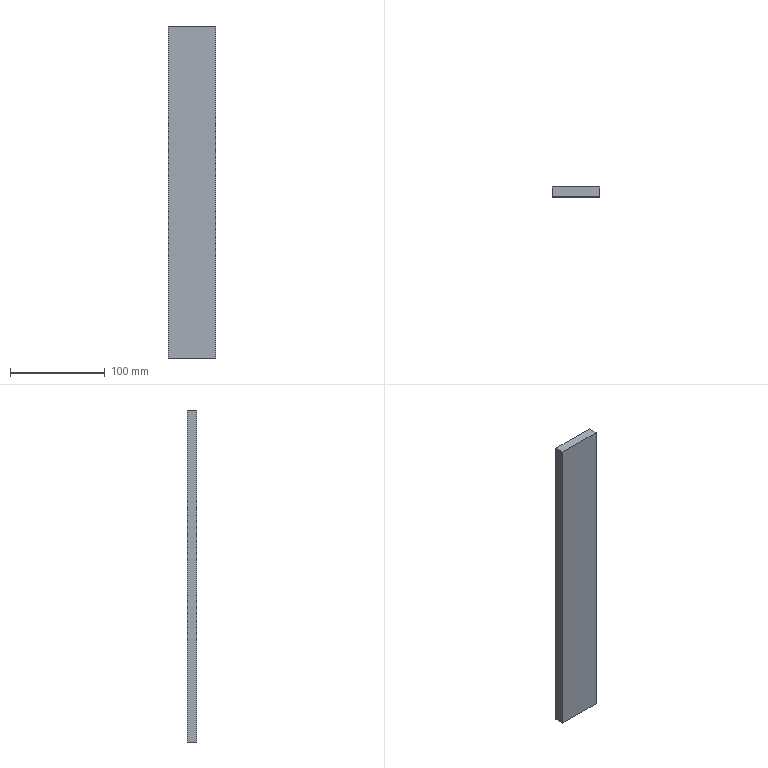Part | NX | features solid 2 | 1 solid | 6 faces | box 50 x 10 x 350 mm | volume 175000 mm3 | plane 6
STEP:
#1=CARTESIAN_POINT('',(635.,615.,-175.));
#2=VERTEX_POINT('',#1);
#3=CARTESIAN_POINT('',(635.,625.,-175.));
#4=VERTEX_POINT('',#3);
#5=CARTESIAN_POINT('',(635.,615.,-175.));
#6=DIRECTION('',(0.,-1.,0.));
#7=VECTOR('',#6,1000.);
#8=LINE('',#5,#7);
#9=EDGE_CURVE('',#2,#4,#8,.F.);
#10=ORIENTED_EDGE('',*,*,#9,.F.);
#11=CARTESIAN_POINT('',(635.,615.,175.));
#12=VERTEX_POINT('',#11);
#13=CARTESIAN_POINT('',(635.,615.,-165.));
#14=DIRECTION('',(0.,0.,1.));
#15=VECTOR('',#14,1000.);
#16=LINE('',#13,#15);
#17=EDGE_CURVE('',#2,#12,#16,.T.);
#18=ORIENTED_EDGE('',*,*,#17,.T.);
#19=CARTESIAN_POINT('',(635.,625.,175.));
#20=VERTEX_POINT('',#19);
#21=CARTESIAN_POINT('',(635.,615.,175.));
#22=DIRECTION('',(0.,1.,0.));
#23=VECTOR('',#22,1000.);
#24=LINE('',#21,#23);
#25=EDGE_CURVE('',#12,#20,#24,.T.);
#26=ORIENTED_EDGE('',*,*,#25,.T.);
#27=CARTESIAN_POINT('',(635.,625.,-165.));
#28=DIRECTION('',(0.,0.,-1.));
#29=VECTOR('',#28,1000.);
#30=LINE('',#27,#29);
#31=EDGE_CURVE('',#4,#20,#30,.F.);
#32=ORIENTED_EDGE('',*,*,#31,.F.);
#33=EDGE_LOOP('',(#10,#18,#26,#32));
#34=FACE_BOUND('',#33,.T.);
#35=CARTESIAN_POINT('',(635.,615.,-165.));
#36=DIRECTION('',(-1.,0.,0.));
#37=DIRECTION('',(0.,0.,1.));
#38=AXIS2_PLACEMENT_3D('',#35,#36,#37);
#39=PLANE('',#38);
#40=ADVANCED_FACE('',(#34),#39,.T.);
#41=ORIENTED_EDGE('',*,*,#25,.F.);
#42=CARTESIAN_POINT('',(685.,615.,175.));
#43=VERTEX_POINT('',#42);
#44=CARTESIAN_POINT('',(635.,615.,175.));
#45=DIRECTION('',(1.,0.,0.));
#46=VECTOR('',#45,1000.);
#47=LINE('',#44,#46);
#48=EDGE_CURVE('',#12,#43,#47,.T.);
#49=ORIENTED_EDGE('',*,*,#48,.T.);
#50=CARTESIAN_POINT('',(685.,625.,175.));
#51=VERTEX_POINT('',#50);
#52=CARTESIAN_POINT('',(685.,615.,175.));
#53=DIRECTION('',(0.,-1.,0.));
#54=VECTOR('',#53,1000.);
#55=LINE('',#52,#54);
#56=EDGE_CURVE('',#43,#51,#55,.F.);
#57=ORIENTED_EDGE('',*,*,#56,.T.);
#58=CARTESIAN_POINT('',(635.,625.,175.));
#59=DIRECTION('',(1.,0.,0.));
#60=VECTOR('',#59,1000.);
#61=LINE('',#58,#60);
#62=EDGE_CURVE('',#20,#51,#61,.T.);
#63=ORIENTED_EDGE('',*,*,#62,.F.);
#64=EDGE_LOOP('',(#41,#49,#57,#63));
#65=FACE_BOUND('',#64,.T.);
#66=CARTESIAN_POINT('',(635.,615.,175.));
#67=DIRECTION('',(0.,0.,1.));
#68=DIRECTION('',(1.,0.,0.));
#69=AXIS2_PLACEMENT_3D('',#66,#67,#68);
#70=PLANE('',#69);
#71=ADVANCED_FACE('',(#65),#70,.T.);
#72=ORIENTED_EDGE('',*,*,#56,.F.);
#73=CARTESIAN_POINT('',(685.,615.,-175.));
#74=VERTEX_POINT('',#73);
#75=CARTESIAN_POINT('',(685.,615.,-165.));
#76=DIRECTION('',(0.,0.,1.));
#77=VECTOR('',#76,1000.);
#78=LINE('',#75,#77);
#79=EDGE_CURVE('',#74,#43,#78,.T.);
#80=ORIENTED_EDGE('',*,*,#79,.F.);
#81=CARTESIAN_POINT('',(685.,625.,-175.));
#82=VERTEX_POINT('',#81);
#83=CARTESIAN_POINT('',(685.,615.,-175.));
#84=DIRECTION('',(0.,1.,0.));
#85=VECTOR('',#84,1000.);
#86=LINE('',#83,#85);
#87=EDGE_CURVE('',#74,#82,#86,.T.);
#88=ORIENTED_EDGE('',*,*,#87,.T.);
#89=CARTESIAN_POINT('',(685.,625.,-165.));
#90=DIRECTION('',(0.,0.,-1.));
#91=VECTOR('',#90,1000.);
#92=LINE('',#89,#91);
#93=EDGE_CURVE('',#82,#51,#92,.F.);
#94=ORIENTED_EDGE('',*,*,#93,.T.);
#95=EDGE_LOOP('',(#72,#80,#88,#94));
#96=FACE_BOUND('',#95,.T.);
#97=CARTESIAN_POINT('',(685.,615.,-165.));
#98=DIRECTION('',(-1.,0.,0.));
#99=DIRECTION('',(0.,0.,1.));
#100=AXIS2_PLACEMENT_3D('',#97,#98,#99);
#101=PLANE('',#100);
#102=ADVANCED_FACE('',(#96),#101,.F.);
#103=CARTESIAN_POINT('',(635.,615.,-175.));
#104=DIRECTION('',(-1.,0.,0.));
#105=VECTOR('',#104,1000.);
#106=LINE('',#103,#105);
#107=EDGE_CURVE('',#2,#74,#106,.F.);
#108=ORIENTED_EDGE('',*,*,#107,.F.);
#109=ORIENTED_EDGE('',*,*,#9,.T.);
#110=CARTESIAN_POINT('',(635.,625.,-175.));
#111=DIRECTION('',(-1.,0.,0.));
#112=VECTOR('',#111,1000.);
#113=LINE('',#110,#112);
#114=EDGE_CURVE('',#4,#82,#113,.F.);
#115=ORIENTED_EDGE('',*,*,#114,.T.);
#116=ORIENTED_EDGE('',*,*,#87,.F.);
#117=EDGE_LOOP('',(#108,#109,#115,#116));
#118=FACE_BOUND('',#117,.T.);
#119=CARTESIAN_POINT('',(635.,615.,-175.));
#120=DIRECTION('',(0.,0.,1.));
#121=DIRECTION('',(1.,0.,0.));
#122=AXIS2_PLACEMENT_3D('',#119,#120,#121);
#123=PLANE('',#122);
#124=ADVANCED_FACE('',(#118),#123,.F.);
#125=ORIENTED_EDGE('',*,*,#93,.F.);
#126=ORIENTED_EDGE('',*,*,#114,.F.);
#127=ORIENTED_EDGE('',*,*,#31,.T.);
#128=ORIENTED_EDGE('',*,*,#62,.T.);
#129=EDGE_LOOP('',(#125,#126,#127,#128));
#130=FACE_BOUND('',#129,.T.);
#131=CARTESIAN_POINT('',(635.,625.,-165.));
#132=DIRECTION('',(0.,1.,0.));
#133=DIRECTION('',(0.,0.,-1.));
#134=AXIS2_PLACEMENT_3D('',#131,#132,#133);
#135=PLANE('',#134);
#136=ADVANCED_FACE('',(#130),#135,.T.);
#137=ORIENTED_EDGE('',*,*,#79,.T.);
#138=ORIENTED_EDGE('',*,*,#48,.F.);
#139=ORIENTED_EDGE('',*,*,#17,.F.);
#140=ORIENTED_EDGE('',*,*,#107,.T.);
#141=EDGE_LOOP('',(#137,#138,#139,#140));
#142=FACE_BOUND('',#141,.T.);
#143=CARTESIAN_POINT('',(635.,615.,-165.));
#144=DIRECTION('',(0.,1.,0.));
#145=DIRECTION('',(0.,0.,-1.));
#146=AXIS2_PLACEMENT_3D('',#143,#144,#145);
#147=PLANE('',#146);
#148=ADVANCED_FACE('',(#142),#147,.F.);
#149=CLOSED_SHELL('',(#40,#71,#102,#124,#136,#148));
#150=MANIFOLD_SOLID_BREP('',#149);
#151=(LENGTH_UNIT()NAMED_UNIT(*)SI_UNIT(.MILLI.,.METRE.));
#152=UNCERTAINTY_MEASURE_WITH_UNIT(LENGTH_MEASURE(0.00001),#151,'','');
#153=(NAMED_UNIT(*)PLANE_ANGLE_UNIT()SI_UNIT($,.RADIAN.));
#154=(NAMED_UNIT(*)SI_UNIT($,.STERADIAN.)SOLID_ANGLE_UNIT());
#155=(GEOMETRIC_REPRESENTATION_CONTEXT(3)GLOBAL_UNCERTAINTY_ASSIGNED_CONTEXT((#152))GLOBAL_UNIT_ASSIGNED_CONTEXT((#151,#153,#154))REPRESENTATION_CONTEXT('',''));
#156=ADVANCED_BREP_SHAPE_REPRESENTATION('',(#150),#155);